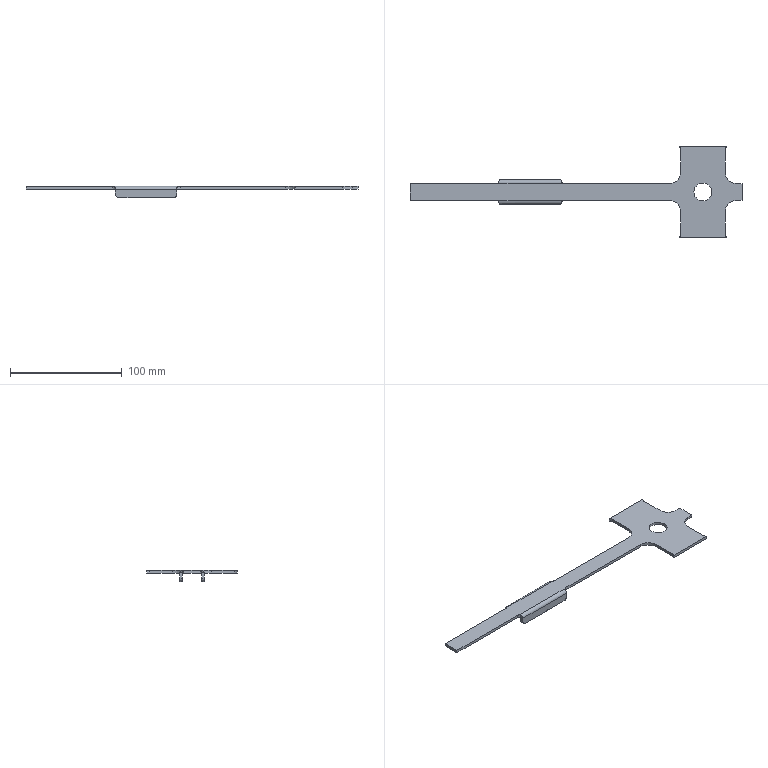Part | STEP file | lll_id950_x_t | 1 solid | 61 faces | box 297 x 81 x 10 mm | volume 20263 mm3 | plane 32 | cylinder 29 | commonest cylinder face diameters 6 x22 20 x4 1 x2 16.1 x1